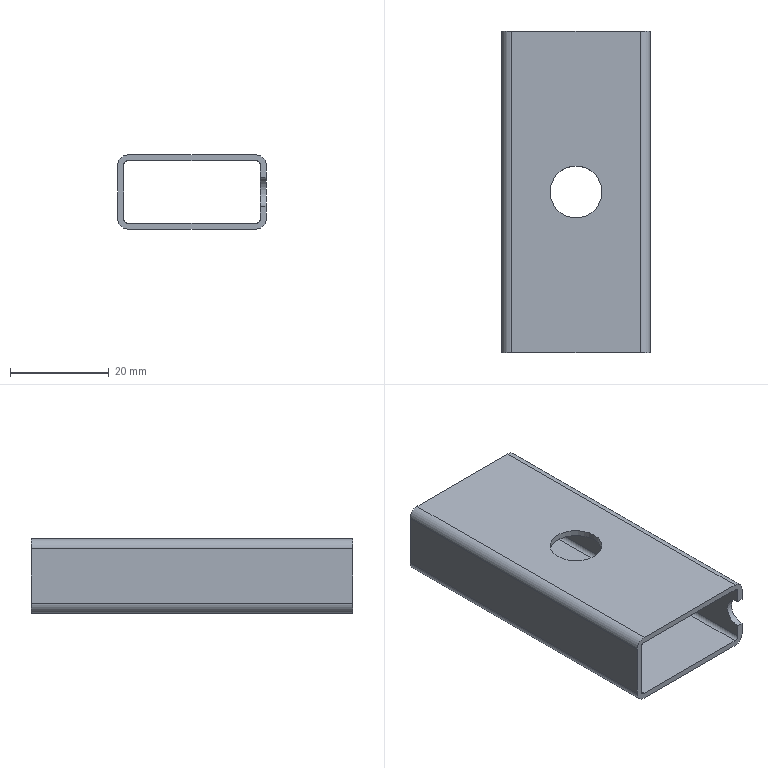Part | STEP file | 7100403 | 1 solid | 22 faces | box 30 x 65 x 15 mm | volume 6216 mm3 | cylinder 12 | plane 10 | commonest cylinder face diameters 1.6 x4 4 x4 6 x2 10.5 x2